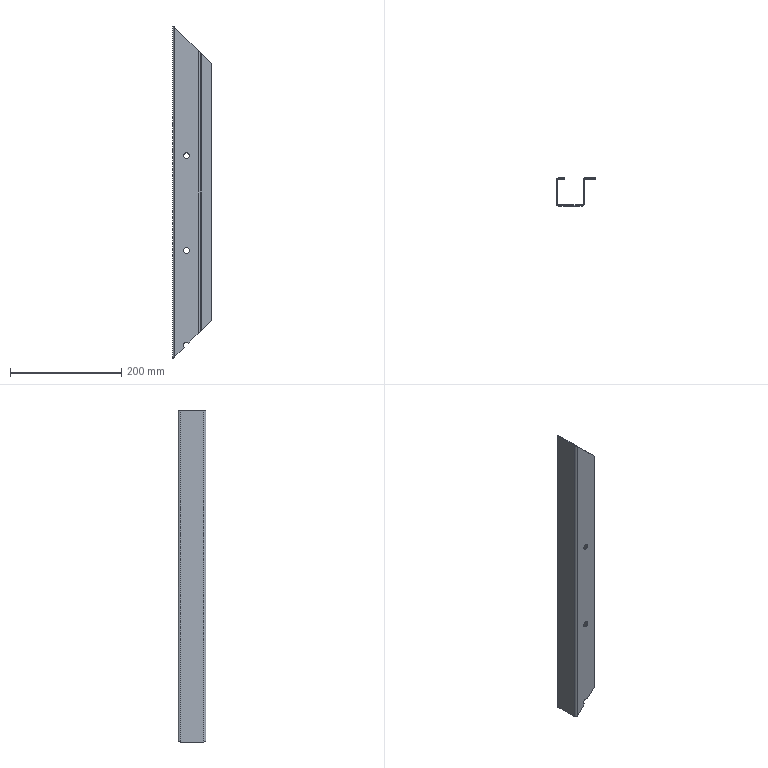Part | STEP file | 750038471 | 1 solid | 44 faces | box 70 x 50 x 596 mm | volume 188466 mm3 | plane 23 | cylinder 13 | spline 8 | commonest cylinder face diameters 10.5 x5 4 x4 8 x4
STEP:
#1=CARTESIAN_POINT('',(25.,2.,70.25));
#2=VERTEX_POINT('',#1);
#3=CARTESIAN_POINT('',(25.,2.,59.75));
#4=VERTEX_POINT('',#3);
#5=CARTESIAN_POINT('',(25.,2.,65.));
#6=DIRECTION('',(0.,-1.,0.));
#7=DIRECTION('',(0.,0.,-1.));
#8=AXIS2_PLACEMENT_3D('',#5,#6,#7);
#9=CIRCLE('',#8,5.25);
#10=EDGE_CURVE('',#2,#4,#9,.T.);
#11=ORIENTED_EDGE('',*,*,#10,.F.);
#12=CARTESIAN_POINT('',(25.,0.,70.25));
#13=VERTEX_POINT('',#12);
#14=CARTESIAN_POINT('',(25.,602.176,70.25));
#15=DIRECTION('',(0.,-1.,0.));
#16=VECTOR('',#15,1000.);
#17=LINE('',#14,#16);
#18=EDGE_CURVE('',#2,#13,#17,.T.);
#19=ORIENTED_EDGE('',*,*,#18,.T.);
#20=CARTESIAN_POINT('',(25.,0.,59.75));
#21=VERTEX_POINT('',#20);
#22=CARTESIAN_POINT('',(25.,0.,65.));
#23=DIRECTION('',(0.,1.,0.));
#24=DIRECTION('',(0.,0.,-1.));
#25=AXIS2_PLACEMENT_3D('',#22,#23,#24);
#26=CIRCLE('',#25,5.25);
#27=EDGE_CURVE('',#21,#13,#26,.T.);
#28=ORIENTED_EDGE('',*,*,#27,.F.);
#29=CARTESIAN_POINT('',(25.,602.176,59.75));
#30=DIRECTION('',(0.,-1.,0.));
#31=VECTOR('',#30,1000.);
#32=LINE('',#29,#31);
#33=EDGE_CURVE('',#4,#21,#32,.T.);
#34=ORIENTED_EDGE('',*,*,#33,.F.);
#35=EDGE_LOOP('',(#11,#19,#28,#34));
#36=FACE_OUTER_BOUND('',#35,.T.);
#37=CARTESIAN_POINT('',(25.,602.176,65.));
#38=DIRECTION('',(0.,-1.,0.));
#39=DIRECTION('',(0.,0.,-1.));
#40=AXIS2_PLACEMENT_3D('',#37,#38,#39);
#41=CYLINDRICAL_SURFACE('',#40,5.25);
#42=ADVANCED_FACE('',(#36),#41,.F.);
#43=CARTESIAN_POINT('',(25.,2.,-99.75));
#44=VERTEX_POINT('',#43);
#45=CARTESIAN_POINT('',(25.,2.,-110.25));
#46=VERTEX_POINT('',#45);
#47=CARTESIAN_POINT('',(25.,2.,-105.));
#48=DIRECTION('',(0.,-1.,0.));
#49=DIRECTION('',(0.,0.,-1.));
#50=AXIS2_PLACEMENT_3D('',#47,#48,#49);
#51=CIRCLE('',#50,5.25);
#52=EDGE_CURVE('',#44,#46,#51,.T.);
#53=ORIENTED_EDGE('',*,*,#52,.F.);
#54=CARTESIAN_POINT('',(25.,0.,-99.75));
#55=VERTEX_POINT('',#54);
#56=CARTESIAN_POINT('',(25.,602.176,-99.75));
#57=DIRECTION('',(0.,-1.,0.));
#58=VECTOR('',#57,1000.);
#59=LINE('',#56,#58);
#60=EDGE_CURVE('',#44,#55,#59,.T.);
#61=ORIENTED_EDGE('',*,*,#60,.T.);
#62=CARTESIAN_POINT('',(25.,0.,-110.25));
#63=VERTEX_POINT('',#62);
#64=CARTESIAN_POINT('',(25.,0.,-105.));
#65=DIRECTION('',(0.,1.,0.));
#66=DIRECTION('',(0.,0.,-1.));
#67=AXIS2_PLACEMENT_3D('',#64,#65,#66);
#68=CIRCLE('',#67,5.25);
#69=EDGE_CURVE('',#63,#55,#68,.T.);
#70=ORIENTED_EDGE('',*,*,#69,.F.);
#71=CARTESIAN_POINT('',(25.,602.176,-110.25));
#72=DIRECTION('',(0.,-1.,0.));
#73=VECTOR('',#72,1000.);
#74=LINE('',#71,#73);
#75=EDGE_CURVE('',#46,#63,#74,.T.);
#76=ORIENTED_EDGE('',*,*,#75,.F.);
#77=EDGE_LOOP('',(#53,#61,#70,#76));
#78=FACE_OUTER_BOUND('',#77,.T.);
#79=CARTESIAN_POINT('',(25.,602.176,-105.));
#80=DIRECTION('',(0.,-1.,0.));
#81=DIRECTION('',(0.,0.,-1.));
#82=AXIS2_PLACEMENT_3D('',#79,#80,#81);
#83=CYLINDRICAL_SURFACE('',#82,5.25);
#84=ADVANCED_FACE('',(#78),#83,.F.);
#85=CARTESIAN_POINT('',(0.,46.,-298.));
#86=VERTEX_POINT('',#85);
#87=CARTESIAN_POINT('',(0.,4.,-298.));
#88=VERTEX_POINT('',#87);
#89=CARTESIAN_POINT('',(0.,0.,-298.));
#90=DIRECTION('',(0.,-1.,0.));
#91=VECTOR('',#90,1000.);
#92=LINE('',#89,#91);
#93=EDGE_CURVE('',#86,#88,#92,.T.);
#94=ORIENTED_EDGE('',*,*,#93,.T.);
#95=CARTESIAN_POINT('',(0.,4.,298.));
#96=VERTEX_POINT('',#95);
#97=CARTESIAN_POINT('',(0.,4.,300.));
#98=DIRECTION('',(0.,0.,1.));
#99=VECTOR('',#98,1000.);
#100=LINE('',#97,#99);
#101=EDGE_CURVE('',#88,#96,#100,.T.);
#102=ORIENTED_EDGE('',*,*,#101,.T.);
#103=CARTESIAN_POINT('',(0.,46.,298.));
#104=VERTEX_POINT('',#103);
#105=CARTESIAN_POINT('',(0.,0.,298.));
#106=DIRECTION('',(0.,1.,0.));
#107=VECTOR('',#106,1000.);
#108=LINE('',#105,#107);
#109=EDGE_CURVE('',#96,#104,#108,.T.);
#110=ORIENTED_EDGE('',*,*,#109,.T.);
#111=CARTESIAN_POINT('',(0.,46.,300.));
#112=DIRECTION('',(0.,0.,-1.));
#113=VECTOR('',#112,1000.);
#114=LINE('',#111,#113);
#115=EDGE_CURVE('',#104,#86,#114,.T.);
#116=ORIENTED_EDGE('',*,*,#115,.T.);
#117=EDGE_LOOP('',(#94,#102,#110,#116));
#118=FACE_OUTER_BOUND('',#117,.T.);
#119=CARTESIAN_POINT('',(0.,0.,300.));
#120=DIRECTION('',(-1.,0.,0.));
#121=DIRECTION('',(0.,-1.,0.));
#122=AXIS2_PLACEMENT_3D('',#119,#120,#121);
#123=PLANE('',#122);
#124=ADVANCED_FACE('',(#118),#123,.T.);
#125=CARTESIAN_POINT('',(4.,0.,-296.));
#126=VERTEX_POINT('',#125);
#127=CARTESIAN_POINT('',(0.,4.,-298.));
#128=CARTESIAN_POINT('',(0.,2.,-298.));
#129=CARTESIAN_POINT('',(1.333,0.,-297.333));
#130=CARTESIAN_POINT('',(4.,0.,-296.));
#131=(BOUNDED_CURVE()B_SPLINE_CURVE(3,(#127,#128,#129,#130),.UNSPECIFIED.,.F.,.T.)B_SPLINE_CURVE_WITH_KNOTS((4,4),(0.,0.006692),.UNSPECIFIED.)CURVE()GEOMETRIC_REPRESENTATION_ITEM()RATIONAL_B_SPLINE_CURVE((1.,0.6667,0.5,0.5))REPRESENTATION_ITEM(''));
#132=EDGE_CURVE('',#88,#126,#131,.T.);
#133=ORIENTED_EDGE('',*,*,#132,.T.);
#134=CARTESIAN_POINT('',(4.,0.,296.));
#135=VERTEX_POINT('',#134);
#136=CARTESIAN_POINT('',(4.,0.,300.));
#137=DIRECTION('',(0.,0.,1.));
#138=VECTOR('',#137,1000.);
#139=LINE('',#136,#138);
#140=EDGE_CURVE('',#126,#135,#139,.T.);
#141=ORIENTED_EDGE('',*,*,#140,.T.);
#142=CARTESIAN_POINT('',(4.,0.,296.));
#143=CARTESIAN_POINT('',(1.333,0.,297.333));
#144=CARTESIAN_POINT('',(0.,2.,298.));
#145=CARTESIAN_POINT('',(0.,4.,298.));
#146=(BOUNDED_CURVE()B_SPLINE_CURVE(3,(#142,#143,#144,#145),.UNSPECIFIED.,.F.,.T.)B_SPLINE_CURVE_WITH_KNOTS((4,4),(0.,0.006641),.UNSPECIFIED.)CURVE()GEOMETRIC_REPRESENTATION_ITEM()RATIONAL_B_SPLINE_CURVE((0.5,0.5,0.6667,1.))REPRESENTATION_ITEM(''));
#147=EDGE_CURVE('',#135,#96,#146,.T.);
#148=ORIENTED_EDGE('',*,*,#147,.T.);
#149=ORIENTED_EDGE('',*,*,#101,.F.);
#150=EDGE_LOOP('',(#133,#141,#148,#149));
#151=FACE_OUTER_BOUND('',#150,.T.);
#152=CARTESIAN_POINT('',(4.,4.,300.));
#153=DIRECTION('',(0.,0.,-1.));
#154=DIRECTION('',(-1.,0.,0.));
#155=AXIS2_PLACEMENT_3D('',#152,#153,#154);
#156=CYLINDRICAL_SURFACE('',#155,4.);
#157=ADVANCED_FACE('',(#151),#156,.T.);
#158=CARTESIAN_POINT('',(2.,46.,-298.));
#159=VERTEX_POINT('',#158);
#160=CARTESIAN_POINT('',(2.,46.,-298.));
#161=DIRECTION('',(-1.,0.,0.));
#162=VECTOR('',#161,1000.);
#163=LINE('',#160,#162);
#164=EDGE_CURVE('',#159,#86,#163,.T.);
#165=ORIENTED_EDGE('',*,*,#164,.F.);
#166=CARTESIAN_POINT('',(2.,4.,-298.));
#167=VERTEX_POINT('',#166);
#168=CARTESIAN_POINT('',(2.,0.,-298.));
#169=DIRECTION('',(0.,1.,0.));
#170=VECTOR('',#169,1000.);
#171=LINE('',#168,#170);
#172=EDGE_CURVE('',#167,#159,#171,.T.);
#173=ORIENTED_EDGE('',*,*,#172,.F.);
#174=CARTESIAN_POINT('',(2.,4.,-298.));
#175=DIRECTION('',(1.,0.,0.));
#176=VECTOR('',#175,1000.);
#177=LINE('',#174,#176);
#178=EDGE_CURVE('',#88,#167,#177,.T.);
#179=ORIENTED_EDGE('',*,*,#178,.F.);
#180=ORIENTED_EDGE('',*,*,#93,.F.);
#181=EDGE_LOOP('',(#165,#173,#179,#180));
#182=FACE_OUTER_BOUND('',#181,.T.);
#183=CARTESIAN_POINT('',(2.,0.,-298.));
#184=DIRECTION('',(0.,0.,1.));
#185=DIRECTION('',(0.,-1.,0.));
#186=AXIS2_PLACEMENT_3D('',#183,#184,#185);
#187=PLANE('',#186);
#188=ADVANCED_FACE('',(#182),#187,.F.);
#189=CARTESIAN_POINT('',(4.,50.,-296.));
#190=VERTEX_POINT('',#189);
#191=CARTESIAN_POINT('',(4.,50.,-296.));
#192=CARTESIAN_POINT('',(1.333,50.,-297.333));
#193=CARTESIAN_POINT('',(0.,48.,-298.));
#194=CARTESIAN_POINT('',(0.,46.,-298.));
#195=(BOUNDED_CURVE()B_SPLINE_CURVE(3,(#191,#192,#193,#194),.UNSPECIFIED.,.F.,.F.)B_SPLINE_CURVE_WITH_KNOTS((4,4),(0.,0.006641),.UNSPECIFIED.)CURVE()GEOMETRIC_REPRESENTATION_ITEM()RATIONAL_B_SPLINE_CURVE((0.5,0.5,0.6667,1.))REPRESENTATION_ITEM(''));
#196=EDGE_CURVE('',#190,#86,#195,.T.);
#197=ORIENTED_EDGE('',*,*,#196,.T.);
#198=ORIENTED_EDGE('',*,*,#115,.F.);
#199=CARTESIAN_POINT('',(4.,50.,296.));
#200=VERTEX_POINT('',#199);
#201=CARTESIAN_POINT('',(0.,46.,298.));
#202=CARTESIAN_POINT('',(0.,48.,298.));
#203=CARTESIAN_POINT('',(1.333,50.,297.333));
#204=CARTESIAN_POINT('',(4.,50.,296.));
#205=(BOUNDED_CURVE()B_SPLINE_CURVE(3,(#201,#202,#203,#204),.UNSPECIFIED.,.F.,.F.)B_SPLINE_CURVE_WITH_KNOTS((4,4),(0.,0.006627),.UNSPECIFIED.)CURVE()GEOMETRIC_REPRESENTATION_ITEM()RATIONAL_B_SPLINE_CURVE((1.,0.6667,0.5,0.5))REPRESENTATION_ITEM(''));
#206=EDGE_CURVE('',#104,#200,#205,.T.);
#207=ORIENTED_EDGE('',*,*,#206,.T.);
#208=CARTESIAN_POINT('',(4.,50.,300.));
#209=DIRECTION('',(0.,0.,-1.));
#210=VECTOR('',#209,1000.);
#211=LINE('',#208,#210);
#212=EDGE_CURVE('',#200,#190,#211,.T.);
#213=ORIENTED_EDGE('',*,*,#212,.T.);
#214=EDGE_LOOP('',(#197,#198,#207,#213));
#215=FACE_OUTER_BOUND('',#214,.T.);
#216=CARTESIAN_POINT('',(4.,46.,300.));
#217=DIRECTION('',(0.,0.,-1.));
#218=DIRECTION('',(-1.,0.,0.));
#219=AXIS2_PLACEMENT_3D('',#216,#217,#218);
#220=CYLINDRICAL_SURFACE('',#219,4.);
#221=ADVANCED_FACE('',(#215),#220,.T.);
#222=CARTESIAN_POINT('',(2.,46.,298.));
#223=VERTEX_POINT('',#222);
#224=CARTESIAN_POINT('',(2.,4.,298.));
#225=VERTEX_POINT('',#224);
#226=CARTESIAN_POINT('',(2.,0.,298.));
#227=DIRECTION('',(0.,-1.,0.));
#228=VECTOR('',#227,1000.);
#229=LINE('',#226,#228);
#230=EDGE_CURVE('',#223,#225,#229,.T.);
#231=ORIENTED_EDGE('',*,*,#230,.F.);
#232=CARTESIAN_POINT('',(2.,46.,298.));
#233=DIRECTION('',(1.,0.,0.));
#234=VECTOR('',#233,1000.);
#235=LINE('',#232,#234);
#236=EDGE_CURVE('',#104,#223,#235,.T.);
#237=ORIENTED_EDGE('',*,*,#236,.F.);
#238=ORIENTED_EDGE('',*,*,#109,.F.);
#239=CARTESIAN_POINT('',(2.,4.,298.));
#240=DIRECTION('',(-1.,0.,0.));
#241=VECTOR('',#240,1000.);
#242=LINE('',#239,#241);
#243=EDGE_CURVE('',#225,#96,#242,.T.);
#244=ORIENTED_EDGE('',*,*,#243,.F.);
#245=EDGE_LOOP('',(#231,#237,#238,#244));
#246=FACE_OUTER_BOUND('',#245,.T.);
#247=CARTESIAN_POINT('',(2.,0.,298.));
#248=DIRECTION('',(0.,0.,-1.));
#249=DIRECTION('',(0.,1.,0.));
#250=AXIS2_PLACEMENT_3D('',#247,#248,#249);
#251=PLANE('',#250);
#252=ADVANCED_FACE('',(#246),#251,.F.);
#253=CARTESIAN_POINT('',(46.,0.,254.));
#254=VERTEX_POINT('',#253);
#255=CARTESIAN_POINT('',(46.,0.,254.));
#256=DIRECTION('',(-0.7071,0.,0.7071));
#257=VECTOR('',#256,1000.);
#258=LINE('',#255,#257);
#259=EDGE_CURVE('',#254,#135,#258,.T.);
#260=ORIENTED_EDGE('',*,*,#259,.T.);
#261=ORIENTED_EDGE('',*,*,#140,.F.);
#262=CARTESIAN_POINT('',(21.288,0.,-278.712));
#263=VERTEX_POINT('',#262);
#264=CARTESIAN_POINT('',(4.,0.,-296.));
#265=DIRECTION('',(0.7071,0.,0.7071));
#266=VECTOR('',#265,1000.);
#267=LINE('',#264,#266);
#268=EDGE_CURVE('',#126,#263,#267,.T.);
#269=ORIENTED_EDGE('',*,*,#268,.T.);
#270=CARTESIAN_POINT('',(28.712,0.,-271.288));
#271=VERTEX_POINT('',#270);
#272=CARTESIAN_POINT('',(25.,0.,-275.));
#273=DIRECTION('',(0.,1.,0.));
#274=DIRECTION('',(0.,0.,-1.));
#275=AXIS2_PLACEMENT_3D('',#272,#273,#274);
#276=CIRCLE('',#275,5.25);
#277=EDGE_CURVE('',#263,#271,#276,.T.);
#278=ORIENTED_EDGE('',*,*,#277,.T.);
#279=CARTESIAN_POINT('',(46.,0.,-254.));
#280=VERTEX_POINT('',#279);
#281=CARTESIAN_POINT('',(28.712,0.,-271.288));
#282=DIRECTION('',(0.7071,0.,0.7071));
#283=VECTOR('',#282,1000.);
#284=LINE('',#281,#283);
#285=EDGE_CURVE('',#271,#280,#284,.T.);
#286=ORIENTED_EDGE('',*,*,#285,.T.);
#287=CARTESIAN_POINT('',(46.,0.,300.));
#288=DIRECTION('',(0.,0.,1.));
#289=VECTOR('',#288,1000.);
#290=LINE('',#287,#289);
#291=EDGE_CURVE('',#280,#254,#290,.T.);
#292=ORIENTED_EDGE('',*,*,#291,.T.);
#293=EDGE_LOOP('',(#260,#261,#269,#278,#286,#292));
#294=FACE_OUTER_BOUND('',#293,.T.);
#295=ORIENTED_EDGE('',*,*,#27,.T.);
#296=CARTESIAN_POINT('',(25.,0.,65.));
#297=DIRECTION('',(0.,1.,0.));
#298=DIRECTION('',(0.,0.,-1.));
#299=AXIS2_PLACEMENT_3D('',#296,#297,#298);
#300=CIRCLE('',#299,5.25);
#301=EDGE_CURVE('',#13,#21,#300,.T.);
#302=ORIENTED_EDGE('',*,*,#301,.T.);
#303=EDGE_LOOP('',(#295,#302));
#304=FACE_BOUND('',#303,.T.);
#305=ORIENTED_EDGE('',*,*,#69,.T.);
#306=CARTESIAN_POINT('',(25.,0.,-105.));
#307=DIRECTION('',(0.,1.,0.));
#308=DIRECTION('',(0.,0.,-1.));
#309=AXIS2_PLACEMENT_3D('',#306,#307,#308);
#310=CIRCLE('',#309,5.25);
#311=EDGE_CURVE('',#55,#63,#310,.T.);
#312=ORIENTED_EDGE('',*,*,#311,.T.);
#313=EDGE_LOOP('',(#305,#312));
#314=FACE_BOUND('',#313,.T.);
#315=CARTESIAN_POINT('',(50.,0.,300.));
#316=DIRECTION('',(0.,-1.,0.));
#317=DIRECTION('',(0.,0.,-1.));
#318=AXIS2_PLACEMENT_3D('',#315,#316,#317);
#319=PLANE('',#318);
#320=ADVANCED_FACE('',(#294,#304,#314),#319,.T.);
#321=CARTESIAN_POINT('',(4.,2.,-296.));
#322=VERTEX_POINT('',#321);
#323=CARTESIAN_POINT('',(4.,1.,-296.));
#324=DIRECTION('',(0.,-1.,0.));
#325=VECTOR('',#324,1000.);
#326=LINE('',#323,#325);
#327=EDGE_CURVE('',#322,#126,#326,.T.);
#328=ORIENTED_EDGE('',*,*,#327,.T.);
#329=ORIENTED_EDGE('',*,*,#132,.F.);
#330=ORIENTED_EDGE('',*,*,#178,.T.);
#331=CARTESIAN_POINT('',(2.,4.,-298.));
#332=CARTESIAN_POINT('',(2.,3.,-298.));
#333=CARTESIAN_POINT('',(2.667,2.,-297.333));
#334=CARTESIAN_POINT('',(4.,2.,-296.));
#335=(BOUNDED_CURVE()B_SPLINE_CURVE(3,(#331,#332,#333,#334),.UNSPECIFIED.,.F.,.F.)B_SPLINE_CURVE_WITH_KNOTS((4,4),(0.,0.003854),.UNSPECIFIED.)CURVE()GEOMETRIC_REPRESENTATION_ITEM()RATIONAL_B_SPLINE_CURVE((1.,0.6667,0.5,0.5))REPRESENTATION_ITEM(''));
#336=EDGE_CURVE('',#167,#322,#335,.T.);
#337=ORIENTED_EDGE('',*,*,#336,.T.);
#338=EDGE_LOOP('',(#328,#329,#330,#337));
#339=FACE_OUTER_BOUND('',#338,.T.);
#340=CARTESIAN_POINT('',(0.,4.,-298.));
#341=CARTESIAN_POINT('',(0.6667,4.,-298.));
#342=CARTESIAN_POINT('',(1.333,4.,-298.));
#343=CARTESIAN_POINT('',(2.,4.,-298.));
#344=CARTESIAN_POINT('',(0.,12.,-298.));
#345=CARTESIAN_POINT('',(0.6667,10.667,-298.));
#346=CARTESIAN_POINT('',(1.333,9.333,-298.));
#347=CARTESIAN_POINT('',(2.,8.,-298.));
#348=CARTESIAN_POINT('',(8.,12.,-294.));
#349=CARTESIAN_POINT('',(7.333,10.667,-294.));
#350=CARTESIAN_POINT('',(6.667,9.333,-294.));
#351=CARTESIAN_POINT('',(6.,8.,-294.));
#352=CARTESIAN_POINT('',(8.,4.,-294.));
#353=CARTESIAN_POINT('',(7.333,4.,-294.));
#354=CARTESIAN_POINT('',(6.667,4.,-294.));
#355=CARTESIAN_POINT('',(6.,4.,-294.));
#356=CARTESIAN_POINT('',(8.,-4.,-294.));
#357=CARTESIAN_POINT('',(7.333,-2.667,-294.));
#358=CARTESIAN_POINT('',(6.667,-1.333,-294.));
#359=CARTESIAN_POINT('',(6.,0.,-294.));
#360=CARTESIAN_POINT('',(0.,-4.,-298.));
#361=CARTESIAN_POINT('',(0.6667,-2.667,-298.));
#362=CARTESIAN_POINT('',(1.333,-1.333,-298.));
#363=CARTESIAN_POINT('',(2.,0.,-298.));
#364=CARTESIAN_POINT('',(0.,4.,-298.));
#365=CARTESIAN_POINT('',(0.6667,4.,-298.));
#366=CARTESIAN_POINT('',(1.333,4.,-298.));
#367=CARTESIAN_POINT('',(2.,4.,-298.));
#368=(BOUNDED_SURFACE()B_SPLINE_SURFACE(3,3,((#340,#341,#342,#343),(#344,#345,#346,#347),(#348,#349,#350,#351),(#352,#353,#354,#355),(#356,#357,#358,#359),(#360,#361,#362,#363),(#364,#365,#366,#367)),.UNSPECIFIED.,.T.,.F.,.F.)B_SPLINE_SURFACE_WITH_KNOTS((4,3,4),(4,4),(0.,0.5,1.),(0.,1.),.UNSPECIFIED.)GEOMETRIC_REPRESENTATION_ITEM()RATIONAL_B_SPLINE_SURFACE(((1.,1.,1.,1.),(0.3333,0.3333,0.3333,0.3333),(0.3333,0.3333,0.3333,0.3333),(1.,1.,1.,1.),(0.3333,0.3333,0.3333,0.3333),(0.3333,0.3333,0.3333,0.3333),(1.,1.,1.,1.)))REPRESENTATION_ITEM('')SURFACE());
#369=ADVANCED_FACE('',(#339),#368,.T.);
#370=ORIENTED_EDGE('',*,*,#243,.T.);
#371=ORIENTED_EDGE('',*,*,#147,.F.);
#372=CARTESIAN_POINT('',(4.,2.,296.));
#373=VERTEX_POINT('',#372);
#374=CARTESIAN_POINT('',(4.,1.,296.));
#375=DIRECTION('',(0.,1.,0.));
#376=VECTOR('',#375,1000.);
#377=LINE('',#374,#376);
#378=EDGE_CURVE('',#135,#373,#377,.T.);
#379=ORIENTED_EDGE('',*,*,#378,.T.);
#380=CARTESIAN_POINT('',(4.,2.,296.));
#381=CARTESIAN_POINT('',(2.667,2.,297.333));
#382=CARTESIAN_POINT('',(2.,3.,298.));
#383=CARTESIAN_POINT('',(2.,4.,298.));
#384=(BOUNDED_CURVE()B_SPLINE_CURVE(3,(#380,#381,#382,#383),.UNSPECIFIED.,.F.,.F.)B_SPLINE_CURVE_WITH_KNOTS((4,4),(0.,0.003785),.UNSPECIFIED.)CURVE()GEOMETRIC_REPRESENTATION_ITEM()RATIONAL_B_SPLINE_CURVE((0.5,0.5,0.6667,1.))REPRESENTATION_ITEM(''));
#385=EDGE_CURVE('',#373,#225,#384,.T.);
#386=ORIENTED_EDGE('',*,*,#385,.T.);
#387=EDGE_LOOP('',(#370,#371,#379,#386));
#388=FACE_OUTER_BOUND('',#387,.T.);
#389=CARTESIAN_POINT('',(8.,4.,294.));
#390=CARTESIAN_POINT('',(7.333,4.,294.));
#391=CARTESIAN_POINT('',(6.667,4.,294.));
#392=CARTESIAN_POINT('',(6.,4.,294.));
#393=CARTESIAN_POINT('',(8.,12.,294.));
#394=CARTESIAN_POINT('',(7.333,10.667,294.));
#395=CARTESIAN_POINT('',(6.667,9.333,294.));
#396=CARTESIAN_POINT('',(6.,8.,294.));
#397=CARTESIAN_POINT('',(0.,12.,298.));
#398=CARTESIAN_POINT('',(0.6667,10.667,298.));
#399=CARTESIAN_POINT('',(1.333,9.333,298.));
#400=CARTESIAN_POINT('',(2.,8.,298.));
#401=CARTESIAN_POINT('',(0.,4.,298.));
#402=CARTESIAN_POINT('',(0.6667,4.,298.));
#403=CARTESIAN_POINT('',(1.333,4.,298.));
#404=CARTESIAN_POINT('',(2.,4.,298.));
#405=CARTESIAN_POINT('',(0.,-4.,298.));
#406=CARTESIAN_POINT('',(0.6667,-2.667,298.));
#407=CARTESIAN_POINT('',(1.333,-1.333,298.));
#408=CARTESIAN_POINT('',(2.,0.,298.));
#409=CARTESIAN_POINT('',(8.,-4.,294.));
#410=CARTESIAN_POINT('',(7.333,-2.667,294.));
#411=CARTESIAN_POINT('',(6.667,-1.333,294.));
#412=CARTESIAN_POINT('',(6.,0.,294.));
#413=CARTESIAN_POINT('',(8.,4.,294.));
#414=CARTESIAN_POINT('',(7.333,4.,294.));
#415=CARTESIAN_POINT('',(6.667,4.,294.));
#416=CARTESIAN_POINT('',(6.,4.,294.));
#417=(BOUNDED_SURFACE()B_SPLINE_SURFACE(3,3,((#389,#390,#391,#392),(#393,#394,#395,#396),(#397,#398,#399,#400),(#401,#402,#403,#404),(#405,#406,#407,#408),(#409,#410,#411,#412),(#413,#414,#415,#416)),.UNSPECIFIED.,.T.,.F.,.T.)B_SPLINE_SURFACE_WITH_KNOTS((4,3,4),(4,4),(0.,0.5,1.),(0.,1.),.UNSPECIFIED.)GEOMETRIC_REPRESENTATION_ITEM()RATIONAL_B_SPLINE_SURFACE(((1.,1.,1.,1.),(0.3333,0.3333,0.3333,0.3333),(0.3333,0.3333,0.3333,0.3333),(1.,1.,1.,1.),(0.3333,0.3333,0.3333,0.3333),(0.3333,0.3333,0.3333,0.3333),(1.,1.,1.,1.)))REPRESENTATION_ITEM('')SURFACE());
#418=ADVANCED_FACE('',(#388),#417,.T.);
#419=ORIENTED_EDGE('',*,*,#164,.T.);
#420=ORIENTED_EDGE('',*,*,#196,.F.);
#421=CARTESIAN_POINT('',(4.,48.,-296.));
#422=VERTEX_POINT('',#421);
#423=CARTESIAN_POINT('',(4.,49.,-296.));
#424=DIRECTION('',(0.,-1.,0.));
#425=VECTOR('',#424,1000.);
#426=LINE('',#423,#425);
#427=EDGE_CURVE('',#190,#422,#426,.T.);
#428=ORIENTED_EDGE('',*,*,#427,.T.);
#429=CARTESIAN_POINT('',(4.,48.,-296.));
#430=CARTESIAN_POINT('',(2.667,48.,-297.333));
#431=CARTESIAN_POINT('',(2.,47.,-298.));
#432=CARTESIAN_POINT('',(2.,46.,-298.));
#433=(BOUNDED_CURVE()B_SPLINE_CURVE(3,(#429,#430,#431,#432),.UNSPECIFIED.,.F.,.F.)B_SPLINE_CURVE_WITH_KNOTS((4,4),(0.,0.003785),.UNSPECIFIED.)CURVE()GEOMETRIC_REPRESENTATION_ITEM()RATIONAL_B_SPLINE_CURVE((0.5,0.5,0.6667,1.))REPRESENTATION_ITEM(''));
#434=EDGE_CURVE('',#422,#159,#433,.T.);
#435=ORIENTED_EDGE('',*,*,#434,.T.);
#436=EDGE_LOOP('',(#419,#420,#428,#435));
#437=FACE_OUTER_BOUND('',#436,.T.);
#438=CARTESIAN_POINT('',(0.,46.,-298.));
#439=CARTESIAN_POINT('',(0.6667,46.,-298.));
#440=CARTESIAN_POINT('',(1.333,46.,-298.));
#441=CARTESIAN_POINT('',(2.,46.,-298.));
#442=CARTESIAN_POINT('',(0.,54.,-298.));
#443=CARTESIAN_POINT('',(0.6667,52.667,-298.));
#444=CARTESIAN_POINT('',(1.333,51.333,-298.));
#445=CARTESIAN_POINT('',(2.,50.,-298.));
#446=CARTESIAN_POINT('',(8.,54.,-294.));
#447=CARTESIAN_POINT('',(7.333,52.667,-294.));
#448=CARTESIAN_POINT('',(6.667,51.333,-294.));
#449=CARTESIAN_POINT('',(6.,50.,-294.));
#450=CARTESIAN_POINT('',(8.,46.,-294.));
#451=CARTESIAN_POINT('',(7.333,46.,-294.));
#452=CARTESIAN_POINT('',(6.667,46.,-294.));
#453=CARTESIAN_POINT('',(6.,46.,-294.));
#454=CARTESIAN_POINT('',(8.,38.,-294.));
#455=CARTESIAN_POINT('',(7.333,39.333,-294.));
#456=CARTESIAN_POINT('',(6.667,40.667,-294.));
#457=CARTESIAN_POINT('',(6.,42.,-294.));
#458=CARTESIAN_POINT('',(0.,38.,-298.));
#459=CARTESIAN_POINT('',(0.6667,39.333,-298.));
#460=CARTESIAN_POINT('',(1.333,40.667,-298.));
#461=CARTESIAN_POINT('',(2.,42.,-298.));
#462=CARTESIAN_POINT('',(0.,46.,-298.));
#463=CARTESIAN_POINT('',(0.6667,46.,-298.));
#464=CARTESIAN_POINT('',(1.333,46.,-298.));
#465=CARTESIAN_POINT('',(2.,46.,-298.));
#466=(BOUNDED_SURFACE()B_SPLINE_SURFACE(3,3,((#438,#439,#440,#441),(#442,#443,#444,#445),(#446,#447,#448,#449),(#450,#451,#452,#453),(#454,#455,#456,#457),(#458,#459,#460,#461),(#462,#463,#464,#465)),.UNSPECIFIED.,.T.,.F.,.T.)B_SPLINE_SURFACE_WITH_KNOTS((4,3,4),(4,4),(0.,0.5,1.),(0.,1.),.UNSPECIFIED.)GEOMETRIC_REPRESENTATION_ITEM()RATIONAL_B_SPLINE_SURFACE(((1.,1.,1.,1.),(0.3333,0.3333,0.3333,0.3333),(0.3333,0.3333,0.3333,0.3333),(1.,1.,1.,1.),(0.3333,0.3333,0.3333,0.3333),(0.3333,0.3333,0.3333,0.3333),(1.,1.,1.,1.)))REPRESENTATION_ITEM('')SURFACE());
#467=ADVANCED_FACE('',(#437),#466,.T.);
#468=ORIENTED_EDGE('',*,*,#230,.T.);
#469=CARTESIAN_POINT('',(2.,4.,300.));
#470=DIRECTION('',(0.,0.,1.));
#471=VECTOR('',#470,1000.);
#472=LINE('',#469,#471);
#473=EDGE_CURVE('',#167,#225,#472,.T.);
#474=ORIENTED_EDGE('',*,*,#473,.F.);
#475=ORIENTED_EDGE('',*,*,#172,.T.);
#476=CARTESIAN_POINT('',(2.,46.,300.));
#477=DIRECTION('',(0.,0.,-1.));
#478=VECTOR('',#477,1000.);
#479=LINE('',#476,#478);
#480=EDGE_CURVE('',#223,#159,#479,.T.);
#481=ORIENTED_EDGE('',*,*,#480,.F.);
#482=EDGE_LOOP('',(#468,#474,#475,#481));
#483=FACE_OUTER_BOUND('',#482,.T.);
#484=CARTESIAN_POINT('',(2.,0.,300.));
#485=DIRECTION('',(-1.,0.,0.));
#486=DIRECTION('',(0.,-1.,0.));
#487=AXIS2_PLACEMENT_3D('',#484,#485,#486);
#488=PLANE('',#487);
#489=ADVANCED_FACE('',(#483),#488,.F.);
#490=CARTESIAN_POINT('',(15.,50.,-285.));
#491=VERTEX_POINT('',#490);
#492=CARTESIAN_POINT('',(15.,50.,-285.));
#493=DIRECTION('',(-0.7071,0.,-0.7071));
#494=VECTOR('',#493,1000.);
#495=LINE('',#492,#494);
#496=EDGE_CURVE('',#491,#190,#495,.T.);
#497=ORIENTED_EDGE('',*,*,#496,.T.);
#498=ORIENTED_EDGE('',*,*,#212,.F.);
#499=CARTESIAN_POINT('',(15.,50.,285.));
#500=VERTEX_POINT('',#499);
#501=CARTESIAN_POINT('',(4.,50.,296.));
#502=DIRECTION('',(0.7071,0.,-0.7071));
#503=VECTOR('',#502,1000.);
#504=LINE('',#501,#503);
#505=EDGE_CURVE('',#200,#500,#504,.T.);
#506=ORIENTED_EDGE('',*,*,#505,.T.);
#507=CARTESIAN_POINT('',(15.,50.,300.));
#508=DIRECTION('',(0.,0.,-1.));
#509=VECTOR('',#508,1000.);
#510=LINE('',#507,#509);
#511=EDGE_CURVE('',#500,#491,#510,.T.);
#512=ORIENTED_EDGE('',*,*,#511,.T.);
#513=EDGE_LOOP('',(#497,#498,#506,#512));
#514=FACE_OUTER_BOUND('',#513,.T.);
#515=CARTESIAN_POINT('',(0.,50.,300.));
#516=DIRECTION('',(0.,1.,0.));
#517=DIRECTION('',(0.,0.,1.));
#518=AXIS2_PLACEMENT_3D('',#515,#516,#517);
#519=PLANE('',#518);
#520=ADVANCED_FACE('',(#514),#519,.T.);
#521=CARTESIAN_POINT('',(4.,48.,296.));
#522=VERTEX_POINT('',#521);
#523=CARTESIAN_POINT('',(4.,49.,296.));
#524=DIRECTION('',(0.,1.,0.));
#525=VECTOR('',#524,1000.);
#526=LINE('',#523,#525);
#527=EDGE_CURVE('',#522,#200,#526,.T.);
#528=ORIENTED_EDGE('',*,*,#527,.T.);
#529=ORIENTED_EDGE('',*,*,#206,.F.);
#530=ORIENTED_EDGE('',*,*,#236,.T.);
#531=CARTESIAN_POINT('',(2.,46.,298.));
#532=CARTESIAN_POINT('',(2.,47.,298.));
#533=CARTESIAN_POINT('',(2.667,48.,297.333));
#534=CARTESIAN_POINT('',(4.,48.,296.));
#535=(BOUNDED_CURVE()B_SPLINE_CURVE(3,(#531,#532,#533,#534),.UNSPECIFIED.,.F.,.F.)B_SPLINE_CURVE_WITH_KNOTS((4,4),(0.,0.003806),.UNSPECIFIED.)CURVE()GEOMETRIC_REPRESENTATION_ITEM()RATIONAL_B_SPLINE_CURVE((1.,0.6667,0.5,0.5))REPRESENTATION_ITEM(''));
#536=EDGE_CURVE('',#223,#522,#535,.T.);
#537=ORIENTED_EDGE('',*,*,#536,.T.);
#538=EDGE_LOOP('',(#528,#529,#530,#537));
#539=FACE_OUTER_BOUND('',#538,.T.);
#540=CARTESIAN_POINT('',(8.,46.,294.));
#541=CARTESIAN_POINT('',(7.333,46.,294.));
#542=CARTESIAN_POINT('',(6.667,46.,294.));
#543=CARTESIAN_POINT('',(6.,46.,294.));
#544=CARTESIAN_POINT('',(8.,54.,294.));
#545=CARTESIAN_POINT('',(7.333,52.667,294.));
#546=CARTESIAN_POINT('',(6.667,51.333,294.));
#547=CARTESIAN_POINT('',(6.,50.,294.));
#548=CARTESIAN_POINT('',(0.,54.,298.));
#549=CARTESIAN_POINT('',(0.6667,52.667,298.));
#550=CARTESIAN_POINT('',(1.333,51.333,298.));
#551=CARTESIAN_POINT('',(2.,50.,298.));
#552=CARTESIAN_POINT('',(0.,46.,298.));
#553=CARTESIAN_POINT('',(0.6667,46.,298.));
#554=CARTESIAN_POINT('',(1.333,46.,298.));
#555=CARTESIAN_POINT('',(2.,46.,298.));
#556=CARTESIAN_POINT('',(0.,38.,298.));
#557=CARTESIAN_POINT('',(0.6667,39.333,298.));
#558=CARTESIAN_POINT('',(1.333,40.667,298.));
#559=CARTESIAN_POINT('',(2.,42.,298.));
#560=CARTESIAN_POINT('',(8.,38.,294.));
#561=CARTESIAN_POINT('',(7.333,39.333,294.));
#562=CARTESIAN_POINT('',(6.667,40.667,294.));
#563=CARTESIAN_POINT('',(6.,42.,294.));
#564=CARTESIAN_POINT('',(8.,46.,294.));
#565=CARTESIAN_POINT('',(7.333,46.,294.));
#566=CARTESIAN_POINT('',(6.667,46.,294.));
#567=CARTESIAN_POINT('',(6.,46.,294.));
#568=(BOUNDED_SURFACE()B_SPLINE_SURFACE(3,3,((#540,#541,#542,#543),(#544,#545,#546,#547),(#548,#549,#550,#551),(#552,#553,#554,#555),(#556,#557,#558,#559),(#560,#561,#562,#563),(#564,#565,#566,#567)),.UNSPECIFIED.,.T.,.F.,.F.)B_SPLINE_SURFACE_WITH_KNOTS((4,3,4),(4,4),(0.,0.5,1.),(0.,1.),.UNSPECIFIED.)GEOMETRIC_REPRESENTATION_ITEM()RATIONAL_B_SPLINE_SURFACE(((1.,1.,1.,1.),(0.3333,0.3333,0.3333,0.3333),(0.3333,0.3333,0.3333,0.3333),(1.,1.,1.,1.),(0.3333,0.3333,0.3333,0.3333),(0.3333,0.3333,0.3333,0.3333),(1.,1.,1.,1.)))REPRESENTATION_ITEM('')SURFACE());
#569=ADVANCED_FACE('',(#539),#568,.T.);
#570=ORIENTED_EDGE('',*,*,#259,.F.);
#571=CARTESIAN_POINT('',(46.,2.,254.));
#572=VERTEX_POINT('',#571);
#573=CARTESIAN_POINT('',(46.,0.,254.));
#574=DIRECTION('',(0.,-1.,0.));
#575=VECTOR('',#574,1000.);
#576=LINE('',#573,#575);
#577=EDGE_CURVE('',#572,#254,#576,.T.);
#578=ORIENTED_EDGE('',*,*,#577,.F.);
#579=CARTESIAN_POINT('',(25.,2.,275.));
#580=DIRECTION('',(0.7071,0.,-0.7071));
#581=VECTOR('',#580,1000.);
#582=LINE('',#579,#581);
#583=EDGE_CURVE('',#373,#572,#582,.T.);
#584=ORIENTED_EDGE('',*,*,#583,.F.);
#585=ORIENTED_EDGE('',*,*,#378,.F.);
#586=EDGE_LOOP('',(#570,#578,#584,#585));
#587=FACE_OUTER_BOUND('',#586,.T.);
#588=CARTESIAN_POINT('',(25.,0.,275.));
#589=DIRECTION('',(-0.7071,0.,-0.7071));
#590=DIRECTION('',(-0.7071,0.,0.7071));
#591=AXIS2_PLACEMENT_3D('',#588,#589,#590);
#592=PLANE('',#591);
#593=ADVANCED_FACE('',(#587),#592,.F.);
#594=CARTESIAN_POINT('',(50.,4.,-250.));
#595=VERTEX_POINT('',#594);
#596=CARTESIAN_POINT('',(46.,0.,-254.));
#597=CARTESIAN_POINT('',(48.667,0.,-251.333));
#598=CARTESIAN_POINT('',(50.,2.,-250.));
#599=CARTESIAN_POINT('',(50.,4.,-250.));
#600=(BOUNDED_CURVE()B_SPLINE_CURVE(3,(#596,#597,#598,#599),.UNSPECIFIED.,.F.,.F.)B_SPLINE_CURVE_WITH_KNOTS((4,4),(0.,0.007567),.UNSPECIFIED.)CURVE()GEOMETRIC_REPRESENTATION_ITEM()RATIONAL_B_SPLINE_CURVE((0.5,0.5,0.6667,1.))REPRESENTATION_ITEM(''));
#601=EDGE_CURVE('',#280,#595,#600,.T.);
#602=ORIENTED_EDGE('',*,*,#601,.T.);
#603=CARTESIAN_POINT('',(50.,4.,250.));
#604=VERTEX_POINT('',#603);
#605=CARTESIAN_POINT('',(50.,4.,300.));
#606=DIRECTION('',(0.,0.,1.));
#607=VECTOR('',#606,1000.);
#608=LINE('',#605,#607);
#609=EDGE_CURVE('',#595,#604,#608,.T.);
#610=ORIENTED_EDGE('',*,*,#609,.T.);
#611=CARTESIAN_POINT('',(50.,4.,250.));
#612=CARTESIAN_POINT('',(50.,2.,250.));
#613=CARTESIAN_POINT('',(48.667,0.,251.333));
#614=CARTESIAN_POINT('',(46.,0.,254.));
#615=(BOUNDED_CURVE()B_SPLINE_CURVE(3,(#611,#612,#613,#614),.UNSPECIFIED.,.F.,.F.)B_SPLINE_CURVE_WITH_KNOTS((4,4),(0.,0.007712),.UNSPECIFIED.)CURVE()GEOMETRIC_REPRESENTATION_ITEM()RATIONAL_B_SPLINE_CURVE((1.,0.6667,0.5,0.5))REPRESENTATION_ITEM(''));
#616=EDGE_CURVE('',#604,#254,#615,.T.);
#617=ORIENTED_EDGE('',*,*,#616,.T.);
#618=ORIENTED_EDGE('',*,*,#291,.F.);
#619=EDGE_LOOP('',(#602,#610,#617,#618));
#620=FACE_OUTER_BOUND('',#619,.T.);
#621=CARTESIAN_POINT('',(46.,4.,300.));
#622=DIRECTION('',(0.,0.,-1.));
#623=DIRECTION('',(-1.,0.,0.));
#624=AXIS2_PLACEMENT_3D('',#621,#622,#623);
#625=CYLINDRICAL_SURFACE('',#624,4.);
#626=ADVANCED_FACE('',(#620),#625,.T.);
#627=CARTESIAN_POINT('',(46.,2.,-254.));
#628=VERTEX_POINT('',#627);
#629=CARTESIAN_POINT('',(28.712,2.,-271.288));
#630=VERTEX_POINT('',#629);
#631=CARTESIAN_POINT('',(325.,2.,25.));
#632=DIRECTION('',(-0.7071,0.,-0.7071));
#633=VECTOR('',#632,1000.);
#634=LINE('',#631,#633);
#635=EDGE_CURVE('',#628,#630,#634,.T.);
#636=ORIENTED_EDGE('',*,*,#635,.F.);
#637=CARTESIAN_POINT('',(46.,0.,-254.));
#638=DIRECTION('',(0.,1.,0.));
#639=VECTOR('',#638,1000.);
#640=LINE('',#637,#639);
#641=EDGE_CURVE('',#280,#628,#640,.T.);
#642=ORIENTED_EDGE('',*,*,#641,.F.);
#643=ORIENTED_EDGE('',*,*,#285,.F.);
#644=CARTESIAN_POINT('',(28.712,0.,-271.288));
#645=DIRECTION('',(0.,-1.,0.));
#646=VECTOR('',#645,1000.);
#647=LINE('',#644,#646);
#648=EDGE_CURVE('',#630,#271,#647,.T.);
#649=ORIENTED_EDGE('',*,*,#648,.F.);
#650=EDGE_LOOP('',(#636,#642,#643,#649));
#651=FACE_OUTER_BOUND('',#650,.T.);
#652=CARTESIAN_POINT('',(325.,0.,25.));
#653=DIRECTION('',(-0.7071,0.,0.7071));
#654=DIRECTION('',(0.7071,0.,0.7071));
#655=AXIS2_PLACEMENT_3D('',#652,#653,#654);
#656=PLANE('',#655);
#657=ADVANCED_FACE('',(#651),#656,.F.);
#658=ORIENTED_EDGE('',*,*,#277,.F.);
#659=CARTESIAN_POINT('',(21.288,2.,-278.712));
#660=VERTEX_POINT('',#659);
#661=CARTESIAN_POINT('',(21.288,0.,-278.712));
#662=DIRECTION('',(0.,-1.,0.));
#663=VECTOR('',#662,1000.);
#664=LINE('',#661,#663);
#665=EDGE_CURVE('',#660,#263,#664,.T.);
#666=ORIENTED_EDGE('',*,*,#665,.F.);
#667=CARTESIAN_POINT('',(25.,2.,-275.));
#668=DIRECTION('',(0.,-1.,0.));
#669=DIRECTION('',(0.,0.,-1.));
#670=AXIS2_PLACEMENT_3D('',#667,#668,#669);
#671=CIRCLE('',#670,5.25);
#672=EDGE_CURVE('',#630,#660,#671,.T.);
#673=ORIENTED_EDGE('',*,*,#672,.F.);
#674=ORIENTED_EDGE('',*,*,#648,.T.);
#675=EDGE_LOOP('',(#658,#666,#673,#674));
#676=FACE_OUTER_BOUND('',#675,.T.);
#677=CARTESIAN_POINT('',(25.,0.,-275.));
#678=DIRECTION('',(0.,-1.,0.));
#679=DIRECTION('',(0.,0.,-1.));
#680=AXIS2_PLACEMENT_3D('',#677,#678,#679);
#681=CYLINDRICAL_SURFACE('',#680,5.25);
#682=ADVANCED_FACE('',(#676),#681,.F.);
#683=ORIENTED_EDGE('',*,*,#665,.T.);
#684=ORIENTED_EDGE('',*,*,#268,.F.);
#685=ORIENTED_EDGE('',*,*,#327,.F.);
#686=CARTESIAN_POINT('',(325.,2.,25.));
#687=DIRECTION('',(-0.7071,0.,-0.7071));
#688=VECTOR('',#687,1000.);
#689=LINE('',#686,#688);
#690=EDGE_CURVE('',#660,#322,#689,.T.);
#691=ORIENTED_EDGE('',*,*,#690,.F.);
#692=EDGE_LOOP('',(#683,#684,#685,#691));
#693=FACE_OUTER_BOUND('',#692,.T.);
#694=CARTESIAN_POINT('',(325.,0.,25.));
#695=DIRECTION('',(-0.7071,0.,0.7071));
#696=DIRECTION('',(0.7071,0.,0.7071));
#697=AXIS2_PLACEMENT_3D('',#694,#695,#696);
#698=PLANE('',#697);
#699=ADVANCED_FACE('',(#693),#698,.F.);
#700=ORIENTED_EDGE('',*,*,#18,.F.);
#701=CARTESIAN_POINT('',(25.,2.,65.));
#702=DIRECTION('',(0.,-1.,0.));
#703=DIRECTION('',(0.,0.,-1.));
#704=AXIS2_PLACEMENT_3D('',#701,#702,#703);
#705=CIRCLE('',#704,5.25);
#706=EDGE_CURVE('',#4,#2,#705,.T.);
#707=ORIENTED_EDGE('',*,*,#706,.F.);
#708=ORIENTED_EDGE('',*,*,#33,.T.);
#709=ORIENTED_EDGE('',*,*,#301,.F.);
#710=EDGE_LOOP('',(#700,#707,#708,#709));
#711=FACE_OUTER_BOUND('',#710,.T.);
#712=CARTESIAN_POINT('',(25.,602.176,65.));
#713=DIRECTION('',(0.,-1.,0.));
#714=DIRECTION('',(0.,0.,-1.));
#715=AXIS2_PLACEMENT_3D('',#712,#713,#714);
#716=CYLINDRICAL_SURFACE('',#715,5.25);
#717=ADVANCED_FACE('',(#711),#716,.F.);
#718=ORIENTED_EDGE('',*,*,#60,.F.);
#719=CARTESIAN_POINT('',(25.,2.,-105.));
#720=DIRECTION('',(0.,-1.,0.));
#721=DIRECTION('',(0.,0.,-1.));
#722=AXIS2_PLACEMENT_3D('',#719,#720,#721);
#723=CIRCLE('',#722,5.25);
#724=EDGE_CURVE('',#46,#44,#723,.T.);
#725=ORIENTED_EDGE('',*,*,#724,.F.);
#726=ORIENTED_EDGE('',*,*,#75,.T.);
#727=ORIENTED_EDGE('',*,*,#311,.F.);
#728=EDGE_LOOP('',(#718,#725,#726,#727));
#729=FACE_OUTER_BOUND('',#728,.T.);
#730=CARTESIAN_POINT('',(25.,602.176,-105.));
#731=DIRECTION('',(0.,-1.,0.));
#732=DIRECTION('',(0.,0.,-1.));
#733=AXIS2_PLACEMENT_3D('',#730,#731,#732);
#734=CYLINDRICAL_SURFACE('',#733,5.25);
#735=ADVANCED_FACE('',(#729),#734,.F.);
#736=ORIENTED_EDGE('',*,*,#385,.F.);
#737=CARTESIAN_POINT('',(4.,2.,300.));
#738=DIRECTION('',(0.,0.,1.));
#739=VECTOR('',#738,1000.);
#740=LINE('',#737,#739);
#741=EDGE_CURVE('',#322,#373,#740,.T.);
#742=ORIENTED_EDGE('',*,*,#741,.F.);
#743=ORIENTED_EDGE('',*,*,#336,.F.);
#744=ORIENTED_EDGE('',*,*,#473,.T.);
#745=EDGE_LOOP('',(#736,#742,#743,#744));
#746=FACE_OUTER_BOUND('',#745,.T.);
#747=CARTESIAN_POINT('',(4.,4.,300.));
#748=DIRECTION('',(0.,0.,-1.));
#749=DIRECTION('',(-1.,0.,0.));
#750=AXIS2_PLACEMENT_3D('',#747,#748,#749);
#751=CYLINDRICAL_SURFACE('',#750,2.);
#752=ADVANCED_FACE('',(#746),#751,.F.);
#753=ORIENTED_EDGE('',*,*,#536,.F.);
#754=ORIENTED_EDGE('',*,*,#480,.T.);
#755=ORIENTED_EDGE('',*,*,#434,.F.);
#756=CARTESIAN_POINT('',(4.,48.,300.));
#757=DIRECTION('',(0.,0.,-1.));
#758=VECTOR('',#757,1000.);
#759=LINE('',#756,#758);
#760=EDGE_CURVE('',#522,#422,#759,.T.);
#761=ORIENTED_EDGE('',*,*,#760,.F.);
#762=EDGE_LOOP('',(#753,#754,#755,#761));
#763=FACE_OUTER_BOUND('',#762,.T.);
#764=CARTESIAN_POINT('',(4.,46.,300.));
#765=DIRECTION('',(0.,0.,-1.));
#766=DIRECTION('',(-1.,0.,0.));
#767=AXIS2_PLACEMENT_3D('',#764,#765,#766);
#768=CYLINDRICAL_SURFACE('',#767,2.);
#769=ADVANCED_FACE('',(#763),#768,.F.);
#770=ORIENTED_EDGE('',*,*,#496,.F.);
#771=CARTESIAN_POINT('',(15.,48.,-285.));
#772=VERTEX_POINT('',#771);
#773=CARTESIAN_POINT('',(15.,50.,-285.));
#774=DIRECTION('',(0.,1.,0.));
#775=VECTOR('',#774,1000.);
#776=LINE('',#773,#775);
#777=EDGE_CURVE('',#772,#491,#776,.T.);
#778=ORIENTED_EDGE('',*,*,#777,.F.);
#779=CARTESIAN_POINT('',(300.,48.,0.));
#780=DIRECTION('',(0.7071,0.,0.7071));
#781=VECTOR('',#780,1000.);
#782=LINE('',#779,#781);
#783=EDGE_CURVE('',#422,#772,#782,.T.);
#784=ORIENTED_EDGE('',*,*,#783,.F.);
#785=ORIENTED_EDGE('',*,*,#427,.F.);
#786=EDGE_LOOP('',(#770,#778,#784,#785));
#787=FACE_OUTER_BOUND('',#786,.T.);
#788=CARTESIAN_POINT('',(300.,50.,0.));
#789=DIRECTION('',(-0.7071,0.,0.7071));
#790=DIRECTION('',(0.7071,0.,0.7071));
#791=AXIS2_PLACEMENT_3D('',#788,#789,#790);
#792=PLANE('',#791);
#793=ADVANCED_FACE('',(#787),#792,.F.);
#794=ORIENTED_EDGE('',*,*,#777,.T.);
#795=ORIENTED_EDGE('',*,*,#511,.F.);
#796=CARTESIAN_POINT('',(15.,48.,285.));
#797=VERTEX_POINT('',#796);
#798=CARTESIAN_POINT('',(15.,50.,285.));
#799=DIRECTION('',(0.,-1.,0.));
#800=VECTOR('',#799,1000.);
#801=LINE('',#798,#800);
#802=EDGE_CURVE('',#500,#797,#801,.T.);
#803=ORIENTED_EDGE('',*,*,#802,.T.);
#804=CARTESIAN_POINT('',(15.,48.,300.));
#805=DIRECTION('',(0.,0.,-1.));
#806=VECTOR('',#805,1000.);
#807=LINE('',#804,#806);
#808=EDGE_CURVE('',#797,#772,#807,.T.);
#809=ORIENTED_EDGE('',*,*,#808,.T.);
#810=EDGE_LOOP('',(#794,#795,#803,#809));
#811=FACE_OUTER_BOUND('',#810,.T.);
#812=CARTESIAN_POINT('',(15.,50.,300.));
#813=DIRECTION('',(1.,0.,0.));
#814=DIRECTION('',(0.,0.,-1.));
#815=AXIS2_PLACEMENT_3D('',#812,#813,#814);
#816=PLANE('',#815);
#817=ADVANCED_FACE('',(#811),#816,.T.);
#818=ORIENTED_EDGE('',*,*,#505,.F.);
#819=ORIENTED_EDGE('',*,*,#527,.F.);
#820=CARTESIAN_POINT('',(0.,48.,300.));
#821=DIRECTION('',(-0.7071,0.,0.7071));
#822=VECTOR('',#821,1000.);
#823=LINE('',#820,#822);
#824=EDGE_CURVE('',#797,#522,#823,.T.);
#825=ORIENTED_EDGE('',*,*,#824,.F.);
#826=ORIENTED_EDGE('',*,*,#802,.F.);
#827=EDGE_LOOP('',(#818,#819,#825,#826));
#828=FACE_OUTER_BOUND('',#827,.T.);
#829=CARTESIAN_POINT('',(0.,50.,300.));
#830=DIRECTION('',(-0.7071,0.,-0.7071));
#831=DIRECTION('',(-0.7071,0.,0.7071));
#832=AXIS2_PLACEMENT_3D('',#829,#830,#831);
#833=PLANE('',#832);
#834=ADVANCED_FACE('',(#828),#833,.F.);
#835=CARTESIAN_POINT('',(48.,4.,250.));
#836=VERTEX_POINT('',#835);
#837=CARTESIAN_POINT('',(49.,4.,250.));
#838=DIRECTION('',(-1.,0.,0.));
#839=VECTOR('',#838,1000.);
#840=LINE('',#837,#839);
#841=EDGE_CURVE('',#604,#836,#840,.T.);
#842=ORIENTED_EDGE('',*,*,#841,.T.);
#843=CARTESIAN_POINT('',(48.,4.,250.));
#844=CARTESIAN_POINT('',(48.,3.,250.));
#845=CARTESIAN_POINT('',(47.333,2.,251.333));
#846=CARTESIAN_POINT('',(46.,2.,254.));
#847=(BOUNDED_CURVE()B_SPLINE_CURVE(3,(#843,#844,#845,#846),.UNSPECIFIED.,.F.,.F.)B_SPLINE_CURVE_WITH_KNOTS((4,4),(0.,0.00529),.UNSPECIFIED.)CURVE()GEOMETRIC_REPRESENTATION_ITEM()RATIONAL_B_SPLINE_CURVE((1.,0.6667,0.5,0.5))REPRESENTATION_ITEM(''));
#848=EDGE_CURVE('',#836,#572,#847,.T.);
#849=ORIENTED_EDGE('',*,*,#848,.T.);
#850=ORIENTED_EDGE('',*,*,#577,.T.);
#851=ORIENTED_EDGE('',*,*,#616,.F.);
#852=EDGE_LOOP('',(#842,#849,#850,#851));
#853=FACE_OUTER_BOUND('',#852,.T.);
#854=CARTESIAN_POINT('',(50.,4.,250.));
#855=CARTESIAN_POINT('',(49.333,4.,250.));
#856=CARTESIAN_POINT('',(48.667,4.,250.));
#857=CARTESIAN_POINT('',(48.,4.,250.));
#858=CARTESIAN_POINT('',(50.,12.,250.));
#859=CARTESIAN_POINT('',(49.333,10.667,250.));
#860=CARTESIAN_POINT('',(48.667,9.333,250.));
#861=CARTESIAN_POINT('',(48.,8.,250.));
#862=CARTESIAN_POINT('',(42.,12.,258.));
#863=CARTESIAN_POINT('',(42.667,10.667,258.));
#864=CARTESIAN_POINT('',(43.333,9.333,258.));
#865=CARTESIAN_POINT('',(44.,8.,258.));
#866=CARTESIAN_POINT('',(42.,4.,258.));
#867=CARTESIAN_POINT('',(42.667,4.,258.));
#868=CARTESIAN_POINT('',(43.333,4.,258.));
#869=CARTESIAN_POINT('',(44.,4.,258.));
#870=CARTESIAN_POINT('',(42.,-4.,258.));
#871=CARTESIAN_POINT('',(42.667,-2.667,258.));
#872=CARTESIAN_POINT('',(43.333,-1.333,258.));
#873=CARTESIAN_POINT('',(44.,0.,258.));
#874=CARTESIAN_POINT('',(50.,-4.,250.));
#875=CARTESIAN_POINT('',(49.333,-2.667,250.));
#876=CARTESIAN_POINT('',(48.667,-1.333,250.));
#877=CARTESIAN_POINT('',(48.,0.,250.));
#878=CARTESIAN_POINT('',(50.,4.,250.));
#879=CARTESIAN_POINT('',(49.333,4.,250.));
#880=CARTESIAN_POINT('',(48.667,4.,250.));
#881=CARTESIAN_POINT('',(48.,4.,250.));
#882=(BOUNDED_SURFACE()B_SPLINE_SURFACE(3,3,((#854,#855,#856,#857),(#858,#859,#860,#861),(#862,#863,#864,#865),(#866,#867,#868,#869),(#870,#871,#872,#873),(#874,#875,#876,#877),(#878,#879,#880,#881)),.UNSPECIFIED.,.T.,.F.,.F.)B_SPLINE_SURFACE_WITH_KNOTS((4,3,4),(4,4),(0.,0.5,1.),(0.,1.),.UNSPECIFIED.)GEOMETRIC_REPRESENTATION_ITEM()RATIONAL_B_SPLINE_SURFACE(((1.,1.,1.,1.),(0.3333,0.3333,0.3333,0.3333),(0.3333,0.3333,0.3333,0.3333),(1.,1.,1.,1.),(0.3333,0.3333,0.3333,0.3333),(0.3333,0.3333,0.3333,0.3333),(1.,1.,1.,1.)))REPRESENTATION_ITEM('')SURFACE());
#883=ADVANCED_FACE('',(#853),#882,.T.);
#884=ORIENTED_EDGE('',*,*,#690,.T.);
#885=ORIENTED_EDGE('',*,*,#741,.T.);
#886=ORIENTED_EDGE('',*,*,#583,.T.);
#887=CARTESIAN_POINT('',(46.,2.,300.));
#888=DIRECTION('',(0.,0.,1.));
#889=VECTOR('',#888,1000.);
#890=LINE('',#887,#889);
#891=EDGE_CURVE('',#628,#572,#890,.T.);
#892=ORIENTED_EDGE('',*,*,#891,.F.);
#893=ORIENTED_EDGE('',*,*,#635,.T.);
#894=ORIENTED_EDGE('',*,*,#672,.T.);
#895=EDGE_LOOP('',(#884,#885,#886,#892,#893,#894));
#896=FACE_OUTER_BOUND('',#895,.T.);
#897=ORIENTED_EDGE('',*,*,#724,.T.);
#898=ORIENTED_EDGE('',*,*,#52,.T.);
#899=EDGE_LOOP('',(#897,#898));
#900=FACE_BOUND('',#899,.T.);
#901=ORIENTED_EDGE('',*,*,#706,.T.);
#902=ORIENTED_EDGE('',*,*,#10,.T.);
#903=EDGE_LOOP('',(#901,#902));
#904=FACE_BOUND('',#903,.T.);
#905=CARTESIAN_POINT('',(50.,2.,300.));
#906=DIRECTION('',(0.,-1.,0.));
#907=DIRECTION('',(0.,0.,-1.));
#908=AXIS2_PLACEMENT_3D('',#905,#906,#907);
#909=PLANE('',#908);
#910=ADVANCED_FACE('',(#896,#900,#904),#909,.F.);
#911=CARTESIAN_POINT('',(50.,46.,-250.));
#912=VERTEX_POINT('',#911);
#913=CARTESIAN_POINT('',(50.,48.,-250.));
#914=DIRECTION('',(0.,1.,0.));
#915=VECTOR('',#914,1000.);
#916=LINE('',#913,#915);
#917=EDGE_CURVE('',#595,#912,#916,.T.);
#918=ORIENTED_EDGE('',*,*,#917,.T.);
#919=CARTESIAN_POINT('',(50.,46.,250.));
#920=VERTEX_POINT('',#919);
#921=CARTESIAN_POINT('',(50.,46.,300.));
#922=DIRECTION('',(0.,0.,1.));
#923=VECTOR('',#922,1000.);
#924=LINE('',#921,#923);
#925=EDGE_CURVE('',#912,#920,#924,.T.);
#926=ORIENTED_EDGE('',*,*,#925,.T.);
#927=CARTESIAN_POINT('',(50.,48.,250.));
#928=DIRECTION('',(0.,-1.,0.));
#929=VECTOR('',#928,1000.);
#930=LINE('',#927,#929);
#931=EDGE_CURVE('',#920,#604,#930,.T.);
#932=ORIENTED_EDGE('',*,*,#931,.T.);
#933=ORIENTED_EDGE('',*,*,#609,.F.);
#934=EDGE_LOOP('',(#918,#926,#932,#933));
#935=FACE_OUTER_BOUND('',#934,.T.);
#936=CARTESIAN_POINT('',(50.,48.,300.));
#937=DIRECTION('',(1.,0.,0.));
#938=DIRECTION('',(0.,1.,0.));
#939=AXIS2_PLACEMENT_3D('',#936,#937,#938);
#940=PLANE('',#939);
#941=ADVANCED_FACE('',(#935),#940,.T.);
#942=ORIENTED_EDGE('',*,*,#641,.T.);
#943=CARTESIAN_POINT('',(48.,4.,-250.));
#944=VERTEX_POINT('',#943);
#945=CARTESIAN_POINT('',(46.,2.,-254.));
#946=CARTESIAN_POINT('',(47.333,2.,-251.333));
#947=CARTESIAN_POINT('',(48.,3.,-250.));
#948=CARTESIAN_POINT('',(48.,4.,-250.));
#949=(BOUNDED_CURVE()B_SPLINE_CURVE(3,(#945,#946,#947,#948),.UNSPECIFIED.,.F.,.T.)B_SPLINE_CURVE_WITH_KNOTS((4,4),(0.,0.005228),.UNSPECIFIED.)CURVE()GEOMETRIC_REPRESENTATION_ITEM()RATIONAL_B_SPLINE_CURVE((0.5,0.5,0.6667,1.))REPRESENTATION_ITEM(''));
#950=EDGE_CURVE('',#628,#944,#949,.T.);
#951=ORIENTED_EDGE('',*,*,#950,.T.);
#952=CARTESIAN_POINT('',(49.,4.,-250.));
#953=DIRECTION('',(1.,0.,0.));
#954=VECTOR('',#953,1000.);
#955=LINE('',#952,#954);
#956=EDGE_CURVE('',#944,#595,#955,.T.);
#957=ORIENTED_EDGE('',*,*,#956,.T.);
#958=ORIENTED_EDGE('',*,*,#601,.F.);
#959=EDGE_LOOP('',(#942,#951,#957,#958));
#960=FACE_OUTER_BOUND('',#959,.T.);
#961=CARTESIAN_POINT('',(42.,4.,-258.));
#962=CARTESIAN_POINT('',(42.667,4.,-258.));
#963=CARTESIAN_POINT('',(43.333,4.,-258.));
#964=CARTESIAN_POINT('',(44.,4.,-258.));
#965=CARTESIAN_POINT('',(42.,12.,-258.));
#966=CARTESIAN_POINT('',(42.667,10.667,-258.));
#967=CARTESIAN_POINT('',(43.333,9.333,-258.));
#968=CARTESIAN_POINT('',(44.,8.,-258.));
#969=CARTESIAN_POINT('',(50.,12.,-250.));
#970=CARTESIAN_POINT('',(49.333,10.667,-250.));
#971=CARTESIAN_POINT('',(48.667,9.333,-250.));
#972=CARTESIAN_POINT('',(48.,8.,-250.));
#973=CARTESIAN_POINT('',(50.,4.,-250.));
#974=CARTESIAN_POINT('',(49.333,4.,-250.));
#975=CARTESIAN_POINT('',(48.667,4.,-250.));
#976=CARTESIAN_POINT('',(48.,4.,-250.));
#977=CARTESIAN_POINT('',(50.,-4.,-250.));
#978=CARTESIAN_POINT('',(49.333,-2.667,-250.));
#979=CARTESIAN_POINT('',(48.667,-1.333,-250.));
#980=CARTESIAN_POINT('',(48.,0.,-250.));
#981=CARTESIAN_POINT('',(42.,-4.,-258.));
#982=CARTESIAN_POINT('',(42.667,-2.667,-258.));
#983=CARTESIAN_POINT('',(43.333,-1.333,-258.));
#984=CARTESIAN_POINT('',(44.,0.,-258.));
#985=CARTESIAN_POINT('',(42.,4.,-258.));
#986=CARTESIAN_POINT('',(42.667,4.,-258.));
#987=CARTESIAN_POINT('',(43.333,4.,-258.));
#988=CARTESIAN_POINT('',(44.,4.,-258.));
#989=(BOUNDED_SURFACE()B_SPLINE_SURFACE(3,3,((#961,#962,#963,#964),(#965,#966,#967,#968),(#969,#970,#971,#972),(#973,#974,#975,#976),(#977,#978,#979,#980),(#981,#982,#983,#984),(#985,#986,#987,#988)),.UNSPECIFIED.,.T.,.F.,.T.)B_SPLINE_SURFACE_WITH_KNOTS((4,3,4),(4,4),(0.,0.5,1.),(0.,1.),.UNSPECIFIED.)GEOMETRIC_REPRESENTATION_ITEM()RATIONAL_B_SPLINE_SURFACE(((1.,1.,1.,1.),(0.3333,0.3333,0.3333,0.3333),(0.3333,0.3333,0.3333,0.3333),(1.,1.,1.,1.),(0.3333,0.3333,0.3333,0.3333),(0.3333,0.3333,0.3333,0.3333),(1.,1.,1.,1.)))REPRESENTATION_ITEM('')SURFACE());
#990=ADVANCED_FACE('',(#960),#989,.T.);
#991=ORIENTED_EDGE('',*,*,#824,.T.);
#992=ORIENTED_EDGE('',*,*,#760,.T.);
#993=ORIENTED_EDGE('',*,*,#783,.T.);
#994=ORIENTED_EDGE('',*,*,#808,.F.);
#995=EDGE_LOOP('',(#991,#992,#993,#994));
#996=FACE_OUTER_BOUND('',#995,.T.);
#997=CARTESIAN_POINT('',(0.,48.,300.));
#998=DIRECTION('',(0.,1.,0.));
#999=DIRECTION('',(0.,0.,1.));
#1000=AXIS2_PLACEMENT_3D('',#997,#998,#999);
#1001=PLANE('',#1000);
#1002=ADVANCED_FACE('',(#996),#1001,.F.);
#1003=ORIENTED_EDGE('',*,*,#848,.F.);
#1004=CARTESIAN_POINT('',(48.,4.,300.));
#1005=DIRECTION('',(0.,0.,1.));
#1006=VECTOR('',#1005,1000.);
#1007=LINE('',#1004,#1006);
#1008=EDGE_CURVE('',#944,#836,#1007,.T.);
#1009=ORIENTED_EDGE('',*,*,#1008,.F.);
#1010=ORIENTED_EDGE('',*,*,#950,.F.);
#1011=ORIENTED_EDGE('',*,*,#891,.T.);
#1012=EDGE_LOOP('',(#1003,#1009,#1010,#1011));
#1013=FACE_OUTER_BOUND('',#1012,.T.);
#1014=CARTESIAN_POINT('',(46.,4.,300.));
#1015=DIRECTION('',(0.,0.,-1.));
#1016=DIRECTION('',(-1.,0.,0.));
#1017=AXIS2_PLACEMENT_3D('',#1014,#1015,#1016);
#1018=CYLINDRICAL_SURFACE('',#1017,2.);
#1019=ADVANCED_FACE('',(#1013),#1018,.F.);
#1020=ORIENTED_EDGE('',*,*,#931,.F.);
#1021=CARTESIAN_POINT('',(48.,46.,250.));
#1022=VERTEX_POINT('',#1021);
#1023=CARTESIAN_POINT('',(50.,46.,250.));
#1024=DIRECTION('',(1.,0.,0.));
#1025=VECTOR('',#1024,1000.);
#1026=LINE('',#1023,#1025);
#1027=EDGE_CURVE('',#1022,#920,#1026,.T.);
#1028=ORIENTED_EDGE('',*,*,#1027,.F.);
#1029=CARTESIAN_POINT('',(48.,48.,250.));
#1030=DIRECTION('',(0.,1.,0.));
#1031=VECTOR('',#1030,1000.);
#1032=LINE('',#1029,#1031);
#1033=EDGE_CURVE('',#836,#1022,#1032,.T.);
#1034=ORIENTED_EDGE('',*,*,#1033,.F.);
#1035=ORIENTED_EDGE('',*,*,#841,.F.);
#1036=EDGE_LOOP('',(#1020,#1028,#1034,#1035));
#1037=FACE_OUTER_BOUND('',#1036,.T.);
#1038=CARTESIAN_POINT('',(50.,48.,250.));
#1039=DIRECTION('',(0.,0.,-1.));
#1040=DIRECTION('',(0.,1.,0.));
#1041=AXIS2_PLACEMENT_3D('',#1038,#1039,#1040);
#1042=PLANE('',#1041);
#1043=ADVANCED_FACE('',(#1037),#1042,.F.);
#1044=ORIENTED_EDGE('',*,*,#925,.F.);
#1045=CARTESIAN_POINT('',(52.,48.,-248.));
#1046=VERTEX_POINT('',#1045);
#1047=CARTESIAN_POINT('',(52.,48.,-248.));
#1048=CARTESIAN_POINT('',(50.667,48.,-249.333));
#1049=CARTESIAN_POINT('',(50.,47.,-250.));
#1050=CARTESIAN_POINT('',(50.,46.,-250.));
#1051=(BOUNDED_CURVE()B_SPLINE_CURVE(3,(#1047,#1048,#1049,#1050),.UNSPECIFIED.,.F.,.F.)B_SPLINE_CURVE_WITH_KNOTS((4,4),(0.,0.003785),.UNSPECIFIED.)CURVE()GEOMETRIC_REPRESENTATION_ITEM()RATIONAL_B_SPLINE_CURVE((0.5,0.5,0.6667,1.))REPRESENTATION_ITEM(''));
#1052=EDGE_CURVE('',#1046,#912,#1051,.T.);
#1053=ORIENTED_EDGE('',*,*,#1052,.F.);
#1054=CARTESIAN_POINT('',(52.,48.,248.));
#1055=VERTEX_POINT('',#1054);
#1056=CARTESIAN_POINT('',(52.,48.,300.));
#1057=DIRECTION('',(0.,0.,-1.));
#1058=VECTOR('',#1057,1000.);
#1059=LINE('',#1056,#1058);
#1060=EDGE_CURVE('',#1055,#1046,#1059,.T.);
#1061=ORIENTED_EDGE('',*,*,#1060,.F.);
#1062=CARTESIAN_POINT('',(50.,46.,250.));
#1063=CARTESIAN_POINT('',(50.,47.,250.));
#1064=CARTESIAN_POINT('',(50.667,48.,249.333));
#1065=CARTESIAN_POINT('',(52.,48.,248.));
#1066=(BOUNDED_CURVE()B_SPLINE_CURVE(3,(#1062,#1063,#1064,#1065),.UNSPECIFIED.,.F.,.T.)B_SPLINE_CURVE_WITH_KNOTS((4,4),(0.,0.003854),.UNSPECIFIED.)CURVE()GEOMETRIC_REPRESENTATION_ITEM()RATIONAL_B_SPLINE_CURVE((1.,0.6667,0.5,0.5))REPRESENTATION_ITEM(''));
#1067=EDGE_CURVE('',#920,#1055,#1066,.T.);
#1068=ORIENTED_EDGE('',*,*,#1067,.F.);
#1069=EDGE_LOOP('',(#1044,#1053,#1061,#1068));
#1070=FACE_OUTER_BOUND('',#1069,.T.);
#1071=CARTESIAN_POINT('',(52.,46.,300.));
#1072=DIRECTION('',(0.,0.,-1.));
#1073=DIRECTION('',(-1.,0.,0.));
#1074=AXIS2_PLACEMENT_3D('',#1071,#1072,#1073);
#1075=CYLINDRICAL_SURFACE('',#1074,2.);
#1076=ADVANCED_FACE('',(#1070),#1075,.F.);
#1077=ORIENTED_EDGE('',*,*,#917,.F.);
#1078=ORIENTED_EDGE('',*,*,#956,.F.);
#1079=CARTESIAN_POINT('',(48.,46.,-250.));
#1080=VERTEX_POINT('',#1079);
#1081=CARTESIAN_POINT('',(48.,48.,-250.));
#1082=DIRECTION('',(0.,-1.,0.));
#1083=VECTOR('',#1082,1000.);
#1084=LINE('',#1081,#1083);
#1085=EDGE_CURVE('',#1080,#944,#1084,.T.);
#1086=ORIENTED_EDGE('',*,*,#1085,.F.);
#1087=CARTESIAN_POINT('',(50.,46.,-250.));
#1088=DIRECTION('',(-1.,0.,0.));
#1089=VECTOR('',#1088,1000.);
#1090=LINE('',#1087,#1089);
#1091=EDGE_CURVE('',#912,#1080,#1090,.T.);
#1092=ORIENTED_EDGE('',*,*,#1091,.F.);
#1093=EDGE_LOOP('',(#1077,#1078,#1086,#1092));
#1094=FACE_OUTER_BOUND('',#1093,.T.);
#1095=CARTESIAN_POINT('',(50.,48.,-250.));
#1096=DIRECTION('',(0.,0.,1.));
#1097=DIRECTION('',(0.,-1.,0.));
#1098=AXIS2_PLACEMENT_3D('',#1095,#1096,#1097);
#1099=PLANE('',#1098);
#1100=ADVANCED_FACE('',(#1094),#1099,.F.);
#1101=ORIENTED_EDGE('',*,*,#1033,.T.);
#1102=CARTESIAN_POINT('',(48.,46.,300.));
#1103=DIRECTION('',(0.,0.,1.));
#1104=VECTOR('',#1103,1000.);
#1105=LINE('',#1102,#1104);
#1106=EDGE_CURVE('',#1080,#1022,#1105,.T.);
#1107=ORIENTED_EDGE('',*,*,#1106,.F.);
#1108=ORIENTED_EDGE('',*,*,#1085,.T.);
#1109=ORIENTED_EDGE('',*,*,#1008,.T.);
#1110=EDGE_LOOP('',(#1101,#1107,#1108,#1109));
#1111=FACE_OUTER_BOUND('',#1110,.T.);
#1112=CARTESIAN_POINT('',(48.,48.,300.));
#1113=DIRECTION('',(1.,0.,0.));
#1114=DIRECTION('',(0.,1.,0.));
#1115=AXIS2_PLACEMENT_3D('',#1112,#1113,#1114);
#1116=PLANE('',#1115);
#1117=ADVANCED_FACE('',(#1111),#1116,.F.);
#1118=CARTESIAN_POINT('',(52.,50.,248.));
#1119=VERTEX_POINT('',#1118);
#1120=CARTESIAN_POINT('',(52.,49.,248.));
#1121=DIRECTION('',(0.,1.,0.));
#1122=VECTOR('',#1121,1000.);
#1123=LINE('',#1120,#1122);
#1124=EDGE_CURVE('',#1055,#1119,#1123,.T.);
#1125=ORIENTED_EDGE('',*,*,#1124,.T.);
#1126=CARTESIAN_POINT('',(52.,50.,248.));
#1127=CARTESIAN_POINT('',(49.333,50.,249.333));
#1128=CARTESIAN_POINT('',(48.,48.,250.));
#1129=CARTESIAN_POINT('',(48.,46.,250.));
#1130=(BOUNDED_CURVE()B_SPLINE_CURVE(3,(#1126,#1127,#1128,#1129),.UNSPECIFIED.,.F.,.F.)B_SPLINE_CURVE_WITH_KNOTS((4,4),(0.,0.006622),.UNSPECIFIED.)CURVE()GEOMETRIC_REPRESENTATION_ITEM()RATIONAL_B_SPLINE_CURVE((0.5,0.5,0.6667,1.))REPRESENTATION_ITEM(''));
#1131=EDGE_CURVE('',#1119,#1022,#1130,.T.);
#1132=ORIENTED_EDGE('',*,*,#1131,.T.);
#1133=ORIENTED_EDGE('',*,*,#1027,.T.);
#1134=ORIENTED_EDGE('',*,*,#1067,.T.);
#1135=EDGE_LOOP('',(#1125,#1132,#1133,#1134));
#1136=FACE_OUTER_BOUND('',#1135,.T.);
#1137=CARTESIAN_POINT('',(54.,46.,246.));
#1138=CARTESIAN_POINT('',(54.667,46.,246.));
#1139=CARTESIAN_POINT('',(55.333,46.,246.));
#1140=CARTESIAN_POINT('',(56.,46.,246.));
#1141=CARTESIAN_POINT('',(54.,42.,246.));
#1142=CARTESIAN_POINT('',(54.667,40.667,246.));
#1143=CARTESIAN_POINT('',(55.333,39.333,246.));
#1144=CARTESIAN_POINT('',(56.,38.,246.));
#1145=CARTESIAN_POINT('',(50.,42.,250.));
#1146=CARTESIAN_POINT('',(49.333,40.667,250.));
#1147=CARTESIAN_POINT('',(48.667,39.333,250.));
#1148=CARTESIAN_POINT('',(48.,38.,250.));
#1149=CARTESIAN_POINT('',(50.,46.,250.));
#1150=CARTESIAN_POINT('',(49.333,46.,250.));
#1151=CARTESIAN_POINT('',(48.667,46.,250.));
#1152=CARTESIAN_POINT('',(48.,46.,250.));
#1153=CARTESIAN_POINT('',(50.,50.,250.));
#1154=CARTESIAN_POINT('',(49.333,51.333,250.));
#1155=CARTESIAN_POINT('',(48.667,52.667,250.));
#1156=CARTESIAN_POINT('',(48.,54.,250.));
#1157=CARTESIAN_POINT('',(54.,50.,246.));
#1158=CARTESIAN_POINT('',(54.667,51.333,246.));
#1159=CARTESIAN_POINT('',(55.333,52.667,246.));
#1160=CARTESIAN_POINT('',(56.,54.,246.));
#1161=CARTESIAN_POINT('',(54.,46.,246.));
#1162=CARTESIAN_POINT('',(54.667,46.,246.));
#1163=CARTESIAN_POINT('',(55.333,46.,246.));
#1164=CARTESIAN_POINT('',(56.,46.,246.));
#1165=(BOUNDED_SURFACE()B_SPLINE_SURFACE(3,3,((#1137,#1138,#1139,#1140),(#1141,#1142,#1143,#1144),(#1145,#1146,#1147,#1148),(#1149,#1150,#1151,#1152),(#1153,#1154,#1155,#1156),(#1157,#1158,#1159,#1160),(#1161,#1162,#1163,#1164)),.UNSPECIFIED.,.T.,.F.,.F.)B_SPLINE_SURFACE_WITH_KNOTS((4,3,4),(4,4),(0.,0.5,1.),(0.,1.),.UNSPECIFIED.)GEOMETRIC_REPRESENTATION_ITEM()RATIONAL_B_SPLINE_SURFACE(((1.,1.,1.,1.),(0.3333,0.3333,0.3333,0.3333),(0.3333,0.3333,0.3333,0.3333),(1.,1.,1.,1.),(0.3333,0.3333,0.3333,0.3333),(0.3333,0.3333,0.3333,0.3333),(1.,1.,1.,1.)))REPRESENTATION_ITEM('')SURFACE());
#1166=ADVANCED_FACE('',(#1136),#1165,.T.);
#1167=ORIENTED_EDGE('',*,*,#1091,.T.);
#1168=CARTESIAN_POINT('',(52.,50.,-248.));
#1169=VERTEX_POINT('',#1168);
#1170=CARTESIAN_POINT('',(48.,46.,-250.));
#1171=CARTESIAN_POINT('',(48.,48.,-250.));
#1172=CARTESIAN_POINT('',(49.333,50.,-249.333));
#1173=CARTESIAN_POINT('',(52.,50.,-248.));
#1174=(BOUNDED_CURVE()B_SPLINE_CURVE(3,(#1170,#1171,#1172,#1173),.UNSPECIFIED.,.F.,.F.)B_SPLINE_CURVE_WITH_KNOTS((4,4),(0.,0.006696),.UNSPECIFIED.)CURVE()GEOMETRIC_REPRESENTATION_ITEM()RATIONAL_B_SPLINE_CURVE((1.,0.6667,0.5,0.5))REPRESENTATION_ITEM(''));
#1175=EDGE_CURVE('',#1080,#1169,#1174,.T.);
#1176=ORIENTED_EDGE('',*,*,#1175,.T.);
#1177=CARTESIAN_POINT('',(52.,49.,-248.));
#1178=DIRECTION('',(0.,-1.,0.));
#1179=VECTOR('',#1178,1000.);
#1180=LINE('',#1177,#1179);
#1181=EDGE_CURVE('',#1169,#1046,#1180,.T.);
#1182=ORIENTED_EDGE('',*,*,#1181,.T.);
#1183=ORIENTED_EDGE('',*,*,#1052,.T.);
#1184=EDGE_LOOP('',(#1167,#1176,#1182,#1183));
#1185=FACE_OUTER_BOUND('',#1184,.T.);
#1186=CARTESIAN_POINT('',(50.,46.,-250.));
#1187=CARTESIAN_POINT('',(49.333,46.,-250.));
#1188=CARTESIAN_POINT('',(48.667,46.,-250.));
#1189=CARTESIAN_POINT('',(48.,46.,-250.));
#1190=CARTESIAN_POINT('',(50.,42.,-250.));
#1191=CARTESIAN_POINT('',(49.333,40.667,-250.));
#1192=CARTESIAN_POINT('',(48.667,39.333,-250.));
#1193=CARTESIAN_POINT('',(48.,38.,-250.));
#1194=CARTESIAN_POINT('',(54.,42.,-246.));
#1195=CARTESIAN_POINT('',(54.667,40.667,-246.));
#1196=CARTESIAN_POINT('',(55.333,39.333,-246.));
#1197=CARTESIAN_POINT('',(56.,38.,-246.));
#1198=CARTESIAN_POINT('',(54.,46.,-246.));
#1199=CARTESIAN_POINT('',(54.667,46.,-246.));
#1200=CARTESIAN_POINT('',(55.333,46.,-246.));
#1201=CARTESIAN_POINT('',(56.,46.,-246.));
#1202=CARTESIAN_POINT('',(54.,50.,-246.));
#1203=CARTESIAN_POINT('',(54.667,51.333,-246.));
#1204=CARTESIAN_POINT('',(55.333,52.667,-246.));
#1205=CARTESIAN_POINT('',(56.,54.,-246.));
#1206=CARTESIAN_POINT('',(50.,50.,-250.));
#1207=CARTESIAN_POINT('',(49.333,51.333,-250.));
#1208=CARTESIAN_POINT('',(48.667,52.667,-250.));
#1209=CARTESIAN_POINT('',(48.,54.,-250.));
#1210=CARTESIAN_POINT('',(50.,46.,-250.));
#1211=CARTESIAN_POINT('',(49.333,46.,-250.));
#1212=CARTESIAN_POINT('',(48.667,46.,-250.));
#1213=CARTESIAN_POINT('',(48.,46.,-250.));
#1214=(BOUNDED_SURFACE()B_SPLINE_SURFACE(3,3,((#1186,#1187,#1188,#1189),(#1190,#1191,#1192,#1193),(#1194,#1195,#1196,#1197),(#1198,#1199,#1200,#1201),(#1202,#1203,#1204,#1205),(#1206,#1207,#1208,#1209),(#1210,#1211,#1212,#1213)),.UNSPECIFIED.,.T.,.F.,.F.)B_SPLINE_SURFACE_WITH_KNOTS((4,3,4),(4,4),(0.,0.5,1.),(0.,1.),.UNSPECIFIED.)GEOMETRIC_REPRESENTATION_ITEM()RATIONAL_B_SPLINE_SURFACE(((1.,1.,1.,1.),(0.3333,0.3333,0.3333,0.3333),(0.3333,0.3333,0.3333,0.3333),(1.,1.,1.,1.),(0.3333,0.3333,0.3333,0.3333),(0.3333,0.3333,0.3333,0.3333),(1.,1.,1.,1.)))REPRESENTATION_ITEM('')SURFACE());
#1215=ADVANCED_FACE('',(#1185),#1214,.T.);
#1216=CARTESIAN_POINT('',(70.,48.,-230.));
#1217=VERTEX_POINT('',#1216);
#1218=CARTESIAN_POINT('',(52.,48.,-248.));
#1219=DIRECTION('',(0.7071,0.,0.7071));
#1220=VECTOR('',#1219,1000.);
#1221=LINE('',#1218,#1220);
#1222=EDGE_CURVE('',#1046,#1217,#1221,.T.);
#1223=ORIENTED_EDGE('',*,*,#1222,.T.);
#1224=CARTESIAN_POINT('',(70.,48.,230.));
#1225=VERTEX_POINT('',#1224);
#1226=CARTESIAN_POINT('',(70.,48.,300.));
#1227=DIRECTION('',(0.,0.,1.));
#1228=VECTOR('',#1227,1000.);
#1229=LINE('',#1226,#1228);
#1230=EDGE_CURVE('',#1217,#1225,#1229,.T.);
#1231=ORIENTED_EDGE('',*,*,#1230,.T.);
#1232=CARTESIAN_POINT('',(70.,48.,230.));
#1233=DIRECTION('',(-0.7071,0.,0.7071));
#1234=VECTOR('',#1233,1000.);
#1235=LINE('',#1232,#1234);
#1236=EDGE_CURVE('',#1225,#1055,#1235,.T.);
#1237=ORIENTED_EDGE('',*,*,#1236,.T.);
#1238=ORIENTED_EDGE('',*,*,#1060,.T.);
#1239=EDGE_LOOP('',(#1223,#1231,#1237,#1238));
#1240=FACE_OUTER_BOUND('',#1239,.T.);
#1241=CARTESIAN_POINT('',(70.,48.,300.));
#1242=DIRECTION('',(0.,-1.,0.));
#1243=DIRECTION('',(0.,0.,-1.));
#1244=AXIS2_PLACEMENT_3D('',#1241,#1242,#1243);
#1245=PLANE('',#1244);
#1246=ADVANCED_FACE('',(#1240),#1245,.T.);
#1247=CARTESIAN_POINT('',(52.,50.,300.));
#1248=DIRECTION('',(0.,0.,-1.));
#1249=VECTOR('',#1248,1000.);
#1250=LINE('',#1247,#1249);
#1251=EDGE_CURVE('',#1119,#1169,#1250,.T.);
#1252=ORIENTED_EDGE('',*,*,#1251,.T.);
#1253=ORIENTED_EDGE('',*,*,#1175,.F.);
#1254=ORIENTED_EDGE('',*,*,#1106,.T.);
#1255=ORIENTED_EDGE('',*,*,#1131,.F.);
#1256=EDGE_LOOP('',(#1252,#1253,#1254,#1255));
#1257=FACE_OUTER_BOUND('',#1256,.T.);
#1258=CARTESIAN_POINT('',(52.,46.,300.));
#1259=DIRECTION('',(0.,0.,-1.));
#1260=DIRECTION('',(-1.,0.,0.));
#1261=AXIS2_PLACEMENT_3D('',#1258,#1259,#1260);
#1262=CYLINDRICAL_SURFACE('',#1261,4.);
#1263=ADVANCED_FACE('',(#1257),#1262,.T.);
#1264=ORIENTED_EDGE('',*,*,#1124,.F.);
#1265=ORIENTED_EDGE('',*,*,#1236,.F.);
#1266=CARTESIAN_POINT('',(70.,50.,230.));
#1267=VERTEX_POINT('',#1266);
#1268=CARTESIAN_POINT('',(70.,48.,230.));
#1269=DIRECTION('',(0.,-1.,0.));
#1270=VECTOR('',#1269,1000.);
#1271=LINE('',#1268,#1270);
#1272=EDGE_CURVE('',#1267,#1225,#1271,.T.);
#1273=ORIENTED_EDGE('',*,*,#1272,.F.);
#1274=CARTESIAN_POINT('',(35.,50.,265.));
#1275=DIRECTION('',(0.7071,0.,-0.7071));
#1276=VECTOR('',#1275,1000.);
#1277=LINE('',#1274,#1276);
#1278=EDGE_CURVE('',#1119,#1267,#1277,.T.);
#1279=ORIENTED_EDGE('',*,*,#1278,.F.);
#1280=EDGE_LOOP('',(#1264,#1265,#1273,#1279));
#1281=FACE_OUTER_BOUND('',#1280,.T.);
#1282=CARTESIAN_POINT('',(35.,48.,265.));
#1283=DIRECTION('',(-0.7071,0.,-0.7071));
#1284=DIRECTION('',(-0.7071,0.,0.7071));
#1285=AXIS2_PLACEMENT_3D('',#1282,#1283,#1284);
#1286=PLANE('',#1285);
#1287=ADVANCED_FACE('',(#1281),#1286,.F.);
#1288=ORIENTED_EDGE('',*,*,#1222,.F.);
#1289=ORIENTED_EDGE('',*,*,#1181,.F.);
#1290=CARTESIAN_POINT('',(70.,50.,-230.));
#1291=VERTEX_POINT('',#1290);
#1292=CARTESIAN_POINT('',(335.,50.,35.));
#1293=DIRECTION('',(-0.7071,0.,-0.7071));
#1294=VECTOR('',#1293,1000.);
#1295=LINE('',#1292,#1294);
#1296=EDGE_CURVE('',#1291,#1169,#1295,.T.);
#1297=ORIENTED_EDGE('',*,*,#1296,.F.);
#1298=CARTESIAN_POINT('',(70.,48.,-230.));
#1299=DIRECTION('',(0.,1.,0.));
#1300=VECTOR('',#1299,1000.);
#1301=LINE('',#1298,#1300);
#1302=EDGE_CURVE('',#1217,#1291,#1301,.T.);
#1303=ORIENTED_EDGE('',*,*,#1302,.F.);
#1304=EDGE_LOOP('',(#1288,#1289,#1297,#1303));
#1305=FACE_OUTER_BOUND('',#1304,.T.);
#1306=CARTESIAN_POINT('',(335.,48.,35.));
#1307=DIRECTION('',(-0.7071,0.,0.7071));
#1308=DIRECTION('',(0.7071,0.,0.7071));
#1309=AXIS2_PLACEMENT_3D('',#1306,#1307,#1308);
#1310=PLANE('',#1309);
#1311=ADVANCED_FACE('',(#1305),#1310,.F.);
#1312=ORIENTED_EDGE('',*,*,#1272,.T.);
#1313=ORIENTED_EDGE('',*,*,#1230,.F.);
#1314=ORIENTED_EDGE('',*,*,#1302,.T.);
#1315=CARTESIAN_POINT('',(70.,50.,300.));
#1316=DIRECTION('',(0.,0.,-1.));
#1317=VECTOR('',#1316,1000.);
#1318=LINE('',#1315,#1317);
#1319=EDGE_CURVE('',#1267,#1291,#1318,.T.);
#1320=ORIENTED_EDGE('',*,*,#1319,.F.);
#1321=EDGE_LOOP('',(#1312,#1313,#1314,#1320));
#1322=FACE_OUTER_BOUND('',#1321,.T.);
#1323=CARTESIAN_POINT('',(70.,48.,300.));
#1324=DIRECTION('',(-1.,0.,0.));
#1325=DIRECTION('',(0.,0.,1.));
#1326=AXIS2_PLACEMENT_3D('',#1323,#1324,#1325);
#1327=PLANE('',#1326);
#1328=ADVANCED_FACE('',(#1322),#1327,.F.);
#1329=ORIENTED_EDGE('',*,*,#1278,.T.);
#1330=ORIENTED_EDGE('',*,*,#1319,.T.);
#1331=ORIENTED_EDGE('',*,*,#1296,.T.);
#1332=ORIENTED_EDGE('',*,*,#1251,.F.);
#1333=EDGE_LOOP('',(#1329,#1330,#1331,#1332));
#1334=FACE_OUTER_BOUND('',#1333,.T.);
#1335=CARTESIAN_POINT('',(70.,50.,300.));
#1336=DIRECTION('',(0.,-1.,0.));
#1337=DIRECTION('',(0.,0.,-1.));
#1338=AXIS2_PLACEMENT_3D('',#1335,#1336,#1337);
#1339=PLANE('',#1338);
#1340=ADVANCED_FACE('',(#1334),#1339,.F.);
#1341=CLOSED_SHELL('',(#42,#84,#124,#157,#188,#221,#252,#320,#369,#418,#467,#489,#520,#569,#593,#626,#657,#682,#699,#717,#735,#752,#769,#793,#817,#834,#883,#910,#941,#990,#1002,#1019,#1043,#1076,#1100,#1117,#1166,#1215,#1246,#1263,#1287,#1311,#1328,#1340));
#1342=MANIFOLD_SOLID_BREP('',#1341);
#1343=CARTESIAN_POINT('',(0.,0.,0.));
#1344=DIRECTION('',(0.,0.,1.));
#1345=DIRECTION('',(1.,0.,0.));
#1346=AXIS2_PLACEMENT_3D('',#1343,#1344,#1345);
#1347=(LENGTH_UNIT()NAMED_UNIT(*)SI_UNIT(.MILLI.,.METRE.));
#1348=UNCERTAINTY_MEASURE_WITH_UNIT(LENGTH_MEASURE(0.00001),#1347,'','');
#1349=(NAMED_UNIT(*)PLANE_ANGLE_UNIT()SI_UNIT($,.RADIAN.));
#1350=(NAMED_UNIT(*)SI_UNIT($,.STERADIAN.)SOLID_ANGLE_UNIT());
#1351=(GEOMETRIC_REPRESENTATION_CONTEXT(3)GLOBAL_UNCERTAINTY_ASSIGNED_CONTEXT((#1348))GLOBAL_UNIT_ASSIGNED_CONTEXT((#1347,#1349,#1350))REPRESENTATION_CONTEXT('',''));
#1352=ADVANCED_BREP_SHAPE_REPRESENTATION('',(#1342,#1346),#1351);